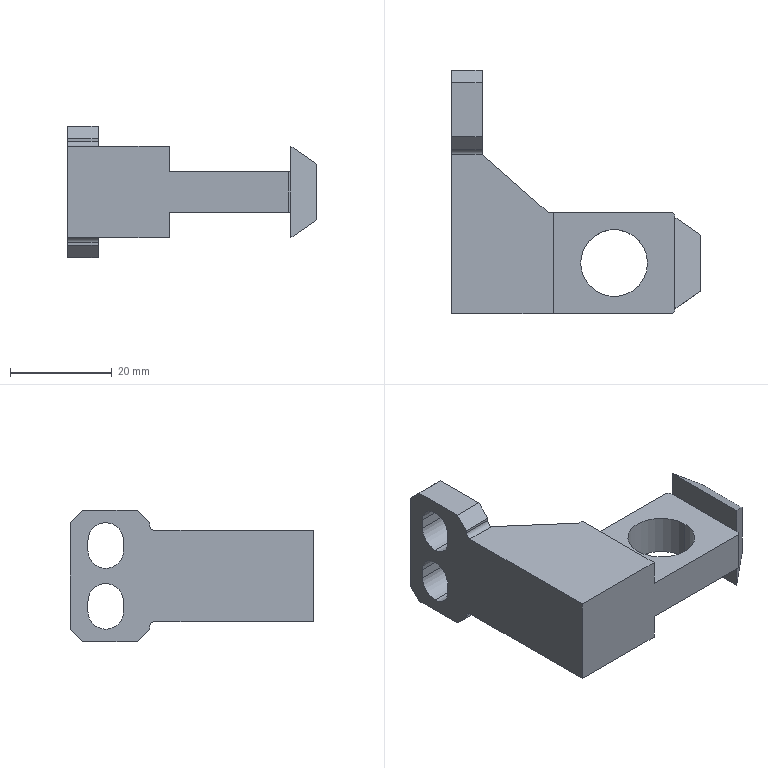Part | SolidWorks | features BaseBody 1 | 1 solid | 51 faces | box 49 x 48 x 26 mm | volume 15129 mm3 | plane 37 | cylinder 14 | commonest cylinder face diameters 7 x6 2 x2 6 x2 8 x2 13.157 x2
STEP:
#1=CARTESIAN_POINT('',(-32.,34.5,-7.));
#2=VERTEX_POINT('',#1);
#3=CARTESIAN_POINT('',(-32.,31.,-10.5));
#4=VERTEX_POINT('',#3);
#5=CARTESIAN_POINT('',(-32.,31.,-7.));
#6=DIRECTION('',(-1.,0.,0.));
#7=DIRECTION('',(0.,0.,-1.));
#8=AXIS2_PLACEMENT_3D('',#5,#6,#7);
#9=CIRCLE('',#8,3.5);
#10=EDGE_CURVE('',#2,#4,#9,.T.);
#11=ORIENTED_EDGE('',*,*,#10,.T.);
#12=CARTESIAN_POINT('',(-26.,31.,-10.5));
#13=VERTEX_POINT('',#12);
#14=CARTESIAN_POINT('',(-26.,31.,-10.5));
#15=DIRECTION('',(1.,0.,0.));
#16=VECTOR('',#15,1000.);
#17=LINE('',#14,#16);
#18=EDGE_CURVE('',#4,#13,#17,.T.);
#19=ORIENTED_EDGE('',*,*,#18,.T.);
#20=CARTESIAN_POINT('',(-26.,34.5,-7.));
#21=VERTEX_POINT('',#20);
#22=CARTESIAN_POINT('',(-26.,31.,-7.));
#23=DIRECTION('',(-1.,0.,0.));
#24=DIRECTION('',(0.,0.,-1.));
#25=AXIS2_PLACEMENT_3D('',#22,#23,#24);
#26=CIRCLE('',#25,3.5);
#27=EDGE_CURVE('',#21,#13,#26,.T.);
#28=ORIENTED_EDGE('',*,*,#27,.F.);
#29=CARTESIAN_POINT('',(-26.,34.5,-7.));
#30=DIRECTION('',(1.,0.,0.));
#31=VECTOR('',#30,1000.);
#32=LINE('',#29,#31);
#33=EDGE_CURVE('',#2,#21,#32,.T.);
#34=ORIENTED_EDGE('',*,*,#33,.F.);
#35=EDGE_LOOP('',(#11,#19,#28,#34));
#36=FACE_OUTER_BOUND('',#35,.T.);
#37=CARTESIAN_POINT('',(-26.,31.,-7.));
#38=DIRECTION('',(1.,0.,0.));
#39=DIRECTION('',(0.,0.,-1.));
#40=AXIS2_PLACEMENT_3D('',#37,#38,#39);
#41=CYLINDRICAL_SURFACE('',#40,3.5);
#42=ADVANCED_FACE('',(#36),#41,.F.);
#43=CARTESIAN_POINT('',(-32.,34.5,5.));
#44=VERTEX_POINT('',#43);
#45=CARTESIAN_POINT('',(-32.,31.,1.5));
#46=VERTEX_POINT('',#45);
#47=CARTESIAN_POINT('',(-32.,31.,5.));
#48=DIRECTION('',(-1.,0.,0.));
#49=DIRECTION('',(0.,0.,-1.));
#50=AXIS2_PLACEMENT_3D('',#47,#48,#49);
#51=CIRCLE('',#50,3.5);
#52=EDGE_CURVE('',#44,#46,#51,.T.);
#53=ORIENTED_EDGE('',*,*,#52,.T.);
#54=CARTESIAN_POINT('',(-26.,31.,1.5));
#55=VERTEX_POINT('',#54);
#56=CARTESIAN_POINT('',(-26.,31.,1.5));
#57=DIRECTION('',(1.,0.,0.));
#58=VECTOR('',#57,1000.);
#59=LINE('',#56,#58);
#60=EDGE_CURVE('',#46,#55,#59,.T.);
#61=ORIENTED_EDGE('',*,*,#60,.T.);
#62=CARTESIAN_POINT('',(-26.,34.5,5.));
#63=VERTEX_POINT('',#62);
#64=CARTESIAN_POINT('',(-26.,31.,5.));
#65=DIRECTION('',(-1.,0.,0.));
#66=DIRECTION('',(0.,0.,-1.));
#67=AXIS2_PLACEMENT_3D('',#64,#65,#66);
#68=CIRCLE('',#67,3.5);
#69=EDGE_CURVE('',#63,#55,#68,.T.);
#70=ORIENTED_EDGE('',*,*,#69,.F.);
#71=CARTESIAN_POINT('',(-26.,34.5,5.));
#72=DIRECTION('',(1.,0.,0.));
#73=VECTOR('',#72,1000.);
#74=LINE('',#71,#73);
#75=EDGE_CURVE('',#44,#63,#74,.T.);
#76=ORIENTED_EDGE('',*,*,#75,.F.);
#77=EDGE_LOOP('',(#53,#61,#70,#76));
#78=FACE_OUTER_BOUND('',#77,.T.);
#79=CARTESIAN_POINT('',(-26.,31.,5.));
#80=DIRECTION('',(1.,0.,0.));
#81=DIRECTION('',(0.,0.,-1.));
#82=AXIS2_PLACEMENT_3D('',#79,#80,#81);
#83=CYLINDRICAL_SURFACE('',#82,3.5);
#84=ADVANCED_FACE('',(#78),#83,.F.);
#85=CARTESIAN_POINT('',(6.579,0.,-4.));
#86=VERTEX_POINT('',#85);
#87=CARTESIAN_POINT('',(-6.579,0.,-4.));
#88=VERTEX_POINT('',#87);
#89=CARTESIAN_POINT('',(0.,0.,-4.));
#90=DIRECTION('',(0.,0.,-1.));
#91=DIRECTION('',(1.,0.,0.));
#92=AXIS2_PLACEMENT_3D('',#89,#90,#91);
#93=CIRCLE('',#92,6.579);
#94=EDGE_CURVE('',#86,#88,#93,.T.);
#95=ORIENTED_EDGE('',*,*,#94,.T.);
#96=CARTESIAN_POINT('',(-6.579,0.,4.));
#97=VERTEX_POINT('',#96);
#98=CARTESIAN_POINT('',(-6.579,0.,-4.));
#99=DIRECTION('',(0.,0.,1.));
#100=VECTOR('',#99,1000.);
#101=LINE('',#98,#100);
#102=EDGE_CURVE('',#88,#97,#101,.T.);
#103=ORIENTED_EDGE('',*,*,#102,.T.);
#104=CARTESIAN_POINT('',(6.579,0.,4.));
#105=VERTEX_POINT('',#104);
#106=CARTESIAN_POINT('',(0.,0.,4.));
#107=DIRECTION('',(0.,0.,-1.));
#108=DIRECTION('',(1.,0.,0.));
#109=AXIS2_PLACEMENT_3D('',#106,#107,#108);
#110=CIRCLE('',#109,6.579);
#111=EDGE_CURVE('',#105,#97,#110,.T.);
#112=ORIENTED_EDGE('',*,*,#111,.F.);
#113=CARTESIAN_POINT('',(6.579,0.,-4.));
#114=DIRECTION('',(0.,0.,1.));
#115=VECTOR('',#114,1000.);
#116=LINE('',#113,#115);
#117=EDGE_CURVE('',#86,#105,#116,.T.);
#118=ORIENTED_EDGE('',*,*,#117,.F.);
#119=EDGE_LOOP('',(#95,#103,#112,#118));
#120=FACE_OUTER_BOUND('',#119,.T.);
#121=CARTESIAN_POINT('',(0.,0.,-4.));
#122=DIRECTION('',(0.,0.,1.));
#123=DIRECTION('',(1.,0.,0.));
#124=AXIS2_PLACEMENT_3D('',#121,#122,#123);
#125=CYLINDRICAL_SURFACE('',#124,6.579);
#126=ADVANCED_FACE('',(#120),#125,.F.);
#127=CARTESIAN_POINT('',(17.,0.,4.));
#128=VERTEX_POINT('',#127);
#129=CARTESIAN_POINT('',(17.,0.,-4.));
#130=VERTEX_POINT('',#129);
#131=CARTESIAN_POINT('',(17.,0.,0.));
#132=DIRECTION('',(1.,0.,0.));
#133=DIRECTION('',(0.,0.,1.));
#134=AXIS2_PLACEMENT_3D('',#131,#132,#133);
#135=CIRCLE('',#134,4.);
#136=EDGE_CURVE('',#128,#130,#135,.T.);
#137=ORIENTED_EDGE('',*,*,#136,.T.);
#138=CARTESIAN_POINT('',(14.,0.,-4.));
#139=VERTEX_POINT('',#138);
#140=CARTESIAN_POINT('',(17.,0.,-4.));
#141=DIRECTION('',(-1.,0.,0.));
#142=VECTOR('',#141,1000.);
#143=LINE('',#140,#142);
#144=EDGE_CURVE('',#130,#139,#143,.T.);
#145=ORIENTED_EDGE('',*,*,#144,.T.);
#146=CARTESIAN_POINT('',(14.,0.,4.));
#147=VERTEX_POINT('',#146);
#148=CARTESIAN_POINT('',(14.,0.,0.));
#149=DIRECTION('',(1.,0.,0.));
#150=DIRECTION('',(0.,0.,1.));
#151=AXIS2_PLACEMENT_3D('',#148,#149,#150);
#152=CIRCLE('',#151,4.);
#153=EDGE_CURVE('',#147,#139,#152,.T.);
#154=ORIENTED_EDGE('',*,*,#153,.F.);
#155=CARTESIAN_POINT('',(17.,0.,4.));
#156=DIRECTION('',(-1.,0.,0.));
#157=VECTOR('',#156,1000.);
#158=LINE('',#155,#157);
#159=EDGE_CURVE('',#128,#147,#158,.T.);
#160=ORIENTED_EDGE('',*,*,#159,.F.);
#161=EDGE_LOOP('',(#137,#145,#154,#160));
#162=FACE_OUTER_BOUND('',#161,.T.);
#163=CARTESIAN_POINT('',(17.,0.,0.));
#164=DIRECTION('',(-1.,0.,0.));
#165=DIRECTION('',(0.,0.,1.));
#166=AXIS2_PLACEMENT_3D('',#163,#164,#165);
#167=CYLINDRICAL_SURFACE('',#166,4.);
#168=ADVANCED_FACE('',(#162),#167,.F.);
#169=CARTESIAN_POINT('',(14.,0.,-3.));
#170=VERTEX_POINT('',#169);
#171=CARTESIAN_POINT('',(14.,0.,3.));
#172=VERTEX_POINT('',#171);
#173=CARTESIAN_POINT('',(14.,0.,0.));
#174=DIRECTION('',(-1.,0.,0.));
#175=DIRECTION('',(0.,0.,1.));
#176=AXIS2_PLACEMENT_3D('',#173,#174,#175);
#177=CIRCLE('',#176,3.);
#178=EDGE_CURVE('',#170,#172,#177,.T.);
#179=ORIENTED_EDGE('',*,*,#178,.F.);
#180=CARTESIAN_POINT('',(9.,0.,-3.));
#181=VERTEX_POINT('',#180);
#182=CARTESIAN_POINT('',(17.,0.,-3.));
#183=DIRECTION('',(-1.,0.,0.));
#184=VECTOR('',#183,1000.);
#185=LINE('',#182,#184);
#186=EDGE_CURVE('',#170,#181,#185,.T.);
#187=ORIENTED_EDGE('',*,*,#186,.T.);
#188=CARTESIAN_POINT('',(9.,0.,3.));
#189=VERTEX_POINT('',#188);
#190=CARTESIAN_POINT('',(9.,0.,0.));
#191=DIRECTION('',(1.,0.,0.));
#192=DIRECTION('',(0.,0.,1.));
#193=AXIS2_PLACEMENT_3D('',#190,#191,#192);
#194=CIRCLE('',#193,3.);
#195=EDGE_CURVE('',#189,#181,#194,.T.);
#196=ORIENTED_EDGE('',*,*,#195,.F.);
#197=CARTESIAN_POINT('',(17.,0.,3.));
#198=DIRECTION('',(-1.,0.,0.));
#199=VECTOR('',#198,1000.);
#200=LINE('',#197,#199);
#201=EDGE_CURVE('',#172,#189,#200,.T.);
#202=ORIENTED_EDGE('',*,*,#201,.F.);
#203=EDGE_LOOP('',(#179,#187,#196,#202));
#204=FACE_OUTER_BOUND('',#203,.T.);
#205=CARTESIAN_POINT('',(17.,0.,0.));
#206=DIRECTION('',(-1.,0.,0.));
#207=DIRECTION('',(0.,0.,1.));
#208=AXIS2_PLACEMENT_3D('',#205,#206,#207);
#209=CYLINDRICAL_SURFACE('',#208,3.);
#210=ADVANCED_FACE('',(#204),#209,.F.);
#211=CARTESIAN_POINT('',(-32.,27.5,-5.));
#212=VERTEX_POINT('',#211);
#213=CARTESIAN_POINT('',(-32.,34.5,-5.));
#214=VERTEX_POINT('',#213);
#215=CARTESIAN_POINT('',(-32.,31.,-5.));
#216=DIRECTION('',(-1.,0.,0.));
#217=DIRECTION('',(0.,0.,-1.));
#218=AXIS2_PLACEMENT_3D('',#215,#216,#217);
#219=CIRCLE('',#218,3.5);
#220=EDGE_CURVE('',#212,#214,#219,.T.);
#221=ORIENTED_EDGE('',*,*,#220,.F.);
#222=CARTESIAN_POINT('',(-32.,27.5,-7.));
#223=VERTEX_POINT('',#222);
#224=CARTESIAN_POINT('',(-32.,27.5,9.));
#225=DIRECTION('',(0.,0.,1.));
#226=VECTOR('',#225,1000.);
#227=LINE('',#224,#226);
#228=EDGE_CURVE('',#223,#212,#227,.T.);
#229=ORIENTED_EDGE('',*,*,#228,.F.);
#230=CARTESIAN_POINT('',(-32.,31.,-7.));
#231=DIRECTION('',(-1.,0.,0.));
#232=DIRECTION('',(0.,0.,-1.));
#233=AXIS2_PLACEMENT_3D('',#230,#231,#232);
#234=CIRCLE('',#233,3.5);
#235=EDGE_CURVE('',#4,#223,#234,.T.);
#236=ORIENTED_EDGE('',*,*,#235,.F.);
#237=ORIENTED_EDGE('',*,*,#10,.F.);
#238=CARTESIAN_POINT('',(-32.,34.5,9.));
#239=DIRECTION('',(0.,0.,-1.));
#240=VECTOR('',#239,1000.);
#241=LINE('',#238,#240);
#242=EDGE_CURVE('',#214,#2,#241,.T.);
#243=ORIENTED_EDGE('',*,*,#242,.F.);
#244=EDGE_LOOP('',(#221,#229,#236,#237,#243));
#245=FACE_BOUND('',#244,.T.);
#246=CARTESIAN_POINT('',(-32.,27.5,7.));
#247=VERTEX_POINT('',#246);
#248=CARTESIAN_POINT('',(-32.,34.5,7.));
#249=VERTEX_POINT('',#248);
#250=CARTESIAN_POINT('',(-32.,31.,7.));
#251=DIRECTION('',(-1.,0.,0.));
#252=DIRECTION('',(0.,0.,-1.));
#253=AXIS2_PLACEMENT_3D('',#250,#251,#252);
#254=CIRCLE('',#253,3.5);
#255=EDGE_CURVE('',#247,#249,#254,.T.);
#256=ORIENTED_EDGE('',*,*,#255,.F.);
#257=CARTESIAN_POINT('',(-32.,27.5,5.));
#258=VERTEX_POINT('',#257);
#259=CARTESIAN_POINT('',(-32.,27.5,9.));
#260=DIRECTION('',(0.,0.,1.));
#261=VECTOR('',#260,1000.);
#262=LINE('',#259,#261);
#263=EDGE_CURVE('',#258,#247,#262,.T.);
#264=ORIENTED_EDGE('',*,*,#263,.F.);
#265=CARTESIAN_POINT('',(-32.,31.,5.));
#266=DIRECTION('',(-1.,0.,0.));
#267=DIRECTION('',(0.,0.,-1.));
#268=AXIS2_PLACEMENT_3D('',#265,#266,#267);
#269=CIRCLE('',#268,3.5);
#270=EDGE_CURVE('',#46,#258,#269,.T.);
#271=ORIENTED_EDGE('',*,*,#270,.F.);
#272=ORIENTED_EDGE('',*,*,#52,.F.);
#273=CARTESIAN_POINT('',(-32.,34.5,9.));
#274=DIRECTION('',(0.,0.,-1.));
#275=VECTOR('',#274,1000.);
#276=LINE('',#273,#275);
#277=EDGE_CURVE('',#249,#44,#276,.T.);
#278=ORIENTED_EDGE('',*,*,#277,.F.);
#279=EDGE_LOOP('',(#256,#264,#271,#272,#278));
#280=FACE_BOUND('',#279,.T.);
#281=CARTESIAN_POINT('',(-32.,-10.,9.));
#282=VERTEX_POINT('',#281);
#283=CARTESIAN_POINT('',(-32.,-10.,-9.));
#284=VERTEX_POINT('',#283);
#285=CARTESIAN_POINT('',(-32.,-10.,9.));
#286=DIRECTION('',(0.,0.,-1.));
#287=VECTOR('',#286,1000.);
#288=LINE('',#285,#287);
#289=EDGE_CURVE('',#282,#284,#288,.T.);
#290=ORIENTED_EDGE('',*,*,#289,.F.);
#291=CARTESIAN_POINT('',(-32.,21.32,9.));
#292=VERTEX_POINT('',#291);
#293=CARTESIAN_POINT('',(-32.,21.32,9.));
#294=DIRECTION('',(0.,-1.,0.));
#295=VECTOR('',#294,1000.);
#296=LINE('',#293,#295);
#297=EDGE_CURVE('',#292,#282,#296,.T.);
#298=ORIENTED_EDGE('',*,*,#297,.F.);
#299=CARTESIAN_POINT('',(-32.,22.32,10.));
#300=VERTEX_POINT('',#299);
#301=CARTESIAN_POINT('',(-32.,21.32,10.));
#302=DIRECTION('',(1.,0.,0.));
#303=DIRECTION('',(0.,0.,-1.));
#304=AXIS2_PLACEMENT_3D('',#301,#302,#303);
#305=CIRCLE('',#304,1.);
#306=EDGE_CURVE('',#292,#300,#305,.T.);
#307=ORIENTED_EDGE('',*,*,#306,.T.);
#308=CARTESIAN_POINT('',(-32.,22.32,10.5));
#309=VERTEX_POINT('',#308);
#310=CARTESIAN_POINT('',(-32.,22.32,10.5));
#311=DIRECTION('',(0.,0.,1.));
#312=VECTOR('',#311,1000.);
#313=LINE('',#310,#312);
#314=EDGE_CURVE('',#300,#309,#313,.T.);
#315=ORIENTED_EDGE('',*,*,#314,.T.);
#316=CARTESIAN_POINT('',(-32.,24.82,13.));
#317=VERTEX_POINT('',#316);
#318=CARTESIAN_POINT('',(-32.,24.82,13.));
#319=DIRECTION('',(0.,-0.7071,-0.7071));
#320=VECTOR('',#319,1000.);
#321=LINE('',#318,#320);
#322=EDGE_CURVE('',#317,#309,#321,.T.);
#323=ORIENTED_EDGE('',*,*,#322,.F.);
#324=CARTESIAN_POINT('',(-32.,35.5,13.));
#325=VERTEX_POINT('',#324);
#326=CARTESIAN_POINT('',(-32.,21.32,13.));
#327=DIRECTION('',(0.,-1.,0.));
#328=VECTOR('',#327,1000.);
#329=LINE('',#326,#328);
#330=EDGE_CURVE('',#325,#317,#329,.T.);
#331=ORIENTED_EDGE('',*,*,#330,.F.);
#332=CARTESIAN_POINT('',(-32.,38.,10.5));
#333=VERTEX_POINT('',#332);
#334=CARTESIAN_POINT('',(-32.,38.,10.5));
#335=DIRECTION('',(0.,-0.7071,0.7071));
#336=VECTOR('',#335,1000.);
#337=LINE('',#334,#336);
#338=EDGE_CURVE('',#333,#325,#337,.T.);
#339=ORIENTED_EDGE('',*,*,#338,.F.);
#340=CARTESIAN_POINT('',(-32.,38.,-10.5));
#341=VERTEX_POINT('',#340);
#342=CARTESIAN_POINT('',(-32.,38.,9.));
#343=DIRECTION('',(0.,0.,1.));
#344=VECTOR('',#343,1000.);
#345=LINE('',#342,#344);
#346=EDGE_CURVE('',#341,#333,#345,.T.);
#347=ORIENTED_EDGE('',*,*,#346,.F.);
#348=CARTESIAN_POINT('',(-32.,35.5,-13.));
#349=VERTEX_POINT('',#348);
#350=CARTESIAN_POINT('',(-32.,35.5,-13.));
#351=DIRECTION('',(0.,0.7071,0.7071));
#352=VECTOR('',#351,1000.);
#353=LINE('',#350,#352);
#354=EDGE_CURVE('',#349,#341,#353,.T.);
#355=ORIENTED_EDGE('',*,*,#354,.F.);
#356=CARTESIAN_POINT('',(-32.,24.82,-13.));
#357=VERTEX_POINT('',#356);
#358=CARTESIAN_POINT('',(-32.,21.32,-13.));
#359=DIRECTION('',(0.,1.,0.));
#360=VECTOR('',#359,1000.);
#361=LINE('',#358,#360);
#362=EDGE_CURVE('',#357,#349,#361,.T.);
#363=ORIENTED_EDGE('',*,*,#362,.F.);
#364=CARTESIAN_POINT('',(-32.,22.32,-10.5));
#365=VERTEX_POINT('',#364);
#366=CARTESIAN_POINT('',(-32.,22.32,-10.5));
#367=DIRECTION('',(0.,0.7071,-0.7071));
#368=VECTOR('',#367,1000.);
#369=LINE('',#366,#368);
#370=EDGE_CURVE('',#365,#357,#369,.T.);
#371=ORIENTED_EDGE('',*,*,#370,.F.);
#372=CARTESIAN_POINT('',(-32.,22.32,-10.));
#373=VERTEX_POINT('',#372);
#374=CARTESIAN_POINT('',(-32.,22.32,-10.));
#375=DIRECTION('',(0.,0.,1.));
#376=VECTOR('',#375,1000.);
#377=LINE('',#374,#376);
#378=EDGE_CURVE('',#365,#373,#377,.T.);
#379=ORIENTED_EDGE('',*,*,#378,.T.);
#380=CARTESIAN_POINT('',(-32.,21.32,-9.));
#381=VERTEX_POINT('',#380);
#382=CARTESIAN_POINT('',(-32.,21.32,-10.));
#383=DIRECTION('',(1.,0.,0.));
#384=DIRECTION('',(0.,0.,-1.));
#385=AXIS2_PLACEMENT_3D('',#382,#383,#384);
#386=CIRCLE('',#385,1.);
#387=EDGE_CURVE('',#373,#381,#386,.T.);
#388=ORIENTED_EDGE('',*,*,#387,.T.);
#389=CARTESIAN_POINT('',(-32.,21.32,-9.));
#390=DIRECTION('',(0.,1.,0.));
#391=VECTOR('',#390,1000.);
#392=LINE('',#389,#391);
#393=EDGE_CURVE('',#284,#381,#392,.T.);
#394=ORIENTED_EDGE('',*,*,#393,.F.);
#395=EDGE_LOOP('',(#290,#298,#307,#315,#323,#331,#339,#347,#355,#363,#371,#379,#388,#394));
#396=FACE_OUTER_BOUND('',#395,.T.);
#397=CARTESIAN_POINT('',(-32.,21.32,9.));
#398=DIRECTION('',(1.,0.,0.));
#399=DIRECTION('',(0.,0.,-1.));
#400=AXIS2_PLACEMENT_3D('',#397,#398,#399);
#401=PLANE('',#400);
#402=ADVANCED_FACE('',(#245,#280,#396),#401,.F.);
#403=CARTESIAN_POINT('',(-26.,34.5,-5.));
#404=VERTEX_POINT('',#403);
#405=CARTESIAN_POINT('',(-26.,34.5,-7.));
#406=DIRECTION('',(0.,0.,1.));
#407=VECTOR('',#406,1000.);
#408=LINE('',#405,#407);
#409=EDGE_CURVE('',#21,#404,#408,.T.);
#410=ORIENTED_EDGE('',*,*,#409,.T.);
#411=CARTESIAN_POINT('',(-26.,34.5,-5.));
#412=DIRECTION('',(-1.,0.,0.));
#413=VECTOR('',#412,1000.);
#414=LINE('',#411,#413);
#415=EDGE_CURVE('',#404,#214,#414,.T.);
#416=ORIENTED_EDGE('',*,*,#415,.T.);
#417=ORIENTED_EDGE('',*,*,#242,.T.);
#418=ORIENTED_EDGE('',*,*,#33,.T.);
#419=EDGE_LOOP('',(#410,#416,#417,#418));
#420=FACE_OUTER_BOUND('',#419,.T.);
#421=CARTESIAN_POINT('',(-26.,34.5,-7.));
#422=DIRECTION('',(0.,-1.,0.));
#423=DIRECTION('',(0.,0.,-1.));
#424=AXIS2_PLACEMENT_3D('',#421,#422,#423);
#425=PLANE('',#424);
#426=ADVANCED_FACE('',(#420),#425,.T.);
#427=ORIENTED_EDGE('',*,*,#415,.F.);
#428=CARTESIAN_POINT('',(-26.,27.5,-5.));
#429=VERTEX_POINT('',#428);
#430=CARTESIAN_POINT('',(-26.,31.,-5.));
#431=DIRECTION('',(-1.,0.,0.));
#432=DIRECTION('',(0.,0.,-1.));
#433=AXIS2_PLACEMENT_3D('',#430,#431,#432);
#434=CIRCLE('',#433,3.5);
#435=EDGE_CURVE('',#429,#404,#434,.T.);
#436=ORIENTED_EDGE('',*,*,#435,.F.);
#437=CARTESIAN_POINT('',(-26.,27.5,-5.));
#438=DIRECTION('',(1.,0.,0.));
#439=VECTOR('',#438,1000.);
#440=LINE('',#437,#439);
#441=EDGE_CURVE('',#212,#429,#440,.T.);
#442=ORIENTED_EDGE('',*,*,#441,.F.);
#443=ORIENTED_EDGE('',*,*,#220,.T.);
#444=EDGE_LOOP('',(#427,#436,#442,#443));
#445=FACE_OUTER_BOUND('',#444,.T.);
#446=CARTESIAN_POINT('',(-26.,31.,-5.));
#447=DIRECTION('',(1.,0.,0.));
#448=DIRECTION('',(0.,0.,-1.));
#449=AXIS2_PLACEMENT_3D('',#446,#447,#448);
#450=CYLINDRICAL_SURFACE('',#449,3.5);
#451=ADVANCED_FACE('',(#445),#450,.F.);
#452=CARTESIAN_POINT('',(-26.,27.5,-7.));
#453=VERTEX_POINT('',#452);
#454=CARTESIAN_POINT('',(-26.,27.5,-5.));
#455=DIRECTION('',(0.,0.,-1.));
#456=VECTOR('',#455,1000.);
#457=LINE('',#454,#456);
#458=EDGE_CURVE('',#429,#453,#457,.T.);
#459=ORIENTED_EDGE('',*,*,#458,.T.);
#460=CARTESIAN_POINT('',(-26.,27.5,-7.));
#461=DIRECTION('',(-1.,0.,0.));
#462=VECTOR('',#461,1000.);
#463=LINE('',#460,#462);
#464=EDGE_CURVE('',#453,#223,#463,.T.);
#465=ORIENTED_EDGE('',*,*,#464,.T.);
#466=ORIENTED_EDGE('',*,*,#228,.T.);
#467=ORIENTED_EDGE('',*,*,#441,.T.);
#468=EDGE_LOOP('',(#459,#465,#466,#467));
#469=FACE_OUTER_BOUND('',#468,.T.);
#470=CARTESIAN_POINT('',(-26.,27.5,-5.));
#471=DIRECTION('',(0.,1.,0.));
#472=DIRECTION('',(0.,0.,1.));
#473=AXIS2_PLACEMENT_3D('',#470,#471,#472);
#474=PLANE('',#473);
#475=ADVANCED_FACE('',(#469),#474,.T.);
#476=ORIENTED_EDGE('',*,*,#18,.F.);
#477=ORIENTED_EDGE('',*,*,#235,.T.);
#478=ORIENTED_EDGE('',*,*,#464,.F.);
#479=CARTESIAN_POINT('',(-26.,31.,-7.));
#480=DIRECTION('',(-1.,0.,0.));
#481=DIRECTION('',(0.,0.,-1.));
#482=AXIS2_PLACEMENT_3D('',#479,#480,#481);
#483=CIRCLE('',#482,3.5);
#484=EDGE_CURVE('',#13,#453,#483,.T.);
#485=ORIENTED_EDGE('',*,*,#484,.F.);
#486=EDGE_LOOP('',(#476,#477,#478,#485));
#487=FACE_OUTER_BOUND('',#486,.T.);
#488=CARTESIAN_POINT('',(-26.,31.,-7.));
#489=DIRECTION('',(1.,0.,0.));
#490=DIRECTION('',(0.,0.,-1.));
#491=AXIS2_PLACEMENT_3D('',#488,#489,#490);
#492=CYLINDRICAL_SURFACE('',#491,3.5);
#493=ADVANCED_FACE('',(#487),#492,.F.);
#494=CARTESIAN_POINT('',(-26.,34.5,7.));
#495=VERTEX_POINT('',#494);
#496=CARTESIAN_POINT('',(-26.,34.5,5.));
#497=DIRECTION('',(0.,0.,1.));
#498=VECTOR('',#497,1000.);
#499=LINE('',#496,#498);
#500=EDGE_CURVE('',#63,#495,#499,.T.);
#501=ORIENTED_EDGE('',*,*,#500,.T.);
#502=CARTESIAN_POINT('',(-26.,34.5,7.));
#503=DIRECTION('',(-1.,0.,0.));
#504=VECTOR('',#503,1000.);
#505=LINE('',#502,#504);
#506=EDGE_CURVE('',#495,#249,#505,.T.);
#507=ORIENTED_EDGE('',*,*,#506,.T.);
#508=ORIENTED_EDGE('',*,*,#277,.T.);
#509=ORIENTED_EDGE('',*,*,#75,.T.);
#510=EDGE_LOOP('',(#501,#507,#508,#509));
#511=FACE_OUTER_BOUND('',#510,.T.);
#512=CARTESIAN_POINT('',(-26.,34.5,5.));
#513=DIRECTION('',(0.,-1.,0.));
#514=DIRECTION('',(0.,0.,-1.));
#515=AXIS2_PLACEMENT_3D('',#512,#513,#514);
#516=PLANE('',#515);
#517=ADVANCED_FACE('',(#511),#516,.T.);
#518=ORIENTED_EDGE('',*,*,#506,.F.);
#519=CARTESIAN_POINT('',(-26.,27.5,7.));
#520=VERTEX_POINT('',#519);
#521=CARTESIAN_POINT('',(-26.,31.,7.));
#522=DIRECTION('',(-1.,0.,0.));
#523=DIRECTION('',(0.,0.,-1.));
#524=AXIS2_PLACEMENT_3D('',#521,#522,#523);
#525=CIRCLE('',#524,3.5);
#526=EDGE_CURVE('',#520,#495,#525,.T.);
#527=ORIENTED_EDGE('',*,*,#526,.F.);
#528=CARTESIAN_POINT('',(-26.,27.5,7.));
#529=DIRECTION('',(1.,0.,0.));
#530=VECTOR('',#529,1000.);
#531=LINE('',#528,#530);
#532=EDGE_CURVE('',#247,#520,#531,.T.);
#533=ORIENTED_EDGE('',*,*,#532,.F.);
#534=ORIENTED_EDGE('',*,*,#255,.T.);
#535=EDGE_LOOP('',(#518,#527,#533,#534));
#536=FACE_OUTER_BOUND('',#535,.T.);
#537=CARTESIAN_POINT('',(-26.,31.,7.));
#538=DIRECTION('',(1.,0.,0.));
#539=DIRECTION('',(0.,0.,-1.));
#540=AXIS2_PLACEMENT_3D('',#537,#538,#539);
#541=CYLINDRICAL_SURFACE('',#540,3.5);
#542=ADVANCED_FACE('',(#536),#541,.F.);
#543=CARTESIAN_POINT('',(-26.,27.5,5.));
#544=VERTEX_POINT('',#543);
#545=CARTESIAN_POINT('',(-26.,27.5,7.));
#546=DIRECTION('',(0.,0.,-1.));
#547=VECTOR('',#546,1000.);
#548=LINE('',#545,#547);
#549=EDGE_CURVE('',#520,#544,#548,.T.);
#550=ORIENTED_EDGE('',*,*,#549,.T.);
#551=CARTESIAN_POINT('',(-26.,27.5,5.));
#552=DIRECTION('',(-1.,0.,0.));
#553=VECTOR('',#552,1000.);
#554=LINE('',#551,#553);
#555=EDGE_CURVE('',#544,#258,#554,.T.);
#556=ORIENTED_EDGE('',*,*,#555,.T.);
#557=ORIENTED_EDGE('',*,*,#263,.T.);
#558=ORIENTED_EDGE('',*,*,#532,.T.);
#559=EDGE_LOOP('',(#550,#556,#557,#558));
#560=FACE_OUTER_BOUND('',#559,.T.);
#561=CARTESIAN_POINT('',(-26.,27.5,7.));
#562=DIRECTION('',(0.,1.,0.));
#563=DIRECTION('',(0.,0.,1.));
#564=AXIS2_PLACEMENT_3D('',#561,#562,#563);
#565=PLANE('',#564);
#566=ADVANCED_FACE('',(#560),#565,.T.);
#567=ORIENTED_EDGE('',*,*,#60,.F.);
#568=ORIENTED_EDGE('',*,*,#270,.T.);
#569=ORIENTED_EDGE('',*,*,#555,.F.);
#570=CARTESIAN_POINT('',(-26.,31.,5.));
#571=DIRECTION('',(-1.,0.,0.));
#572=DIRECTION('',(0.,0.,-1.));
#573=AXIS2_PLACEMENT_3D('',#570,#571,#572);
#574=CIRCLE('',#573,3.5);
#575=EDGE_CURVE('',#55,#544,#574,.T.);
#576=ORIENTED_EDGE('',*,*,#575,.F.);
#577=EDGE_LOOP('',(#567,#568,#569,#576));
#578=FACE_OUTER_BOUND('',#577,.T.);
#579=CARTESIAN_POINT('',(-26.,31.,5.));
#580=DIRECTION('',(1.,0.,0.));
#581=DIRECTION('',(0.,0.,-1.));
#582=AXIS2_PLACEMENT_3D('',#579,#580,#581);
#583=CYLINDRICAL_SURFACE('',#582,3.5);
#584=ADVANCED_FACE('',(#578),#583,.F.);
#585=CARTESIAN_POINT('',(-26.,21.32,-9.));
#586=VERTEX_POINT('',#585);
#587=CARTESIAN_POINT('',(0.,21.32,-9.));
#588=DIRECTION('',(-1.,0.,0.));
#589=VECTOR('',#588,1000.);
#590=LINE('',#587,#589);
#591=EDGE_CURVE('',#586,#381,#590,.T.);
#592=ORIENTED_EDGE('',*,*,#591,.F.);
#593=CARTESIAN_POINT('',(-13.,10.,-9.));
#594=VERTEX_POINT('',#593);
#595=CARTESIAN_POINT('',(-13.,10.,-9.));
#596=DIRECTION('',(-0.7542,0.6567,0.));
#597=VECTOR('',#596,1000.);
#598=LINE('',#595,#597);
#599=EDGE_CURVE('',#594,#586,#598,.T.);
#600=ORIENTED_EDGE('',*,*,#599,.F.);
#601=CARTESIAN_POINT('',(-12.,10.,-9.));
#602=VERTEX_POINT('',#601);
#603=CARTESIAN_POINT('',(11.5,10.,-9.));
#604=DIRECTION('',(1.,0.,0.));
#605=VECTOR('',#604,1000.);
#606=LINE('',#603,#605);
#607=EDGE_CURVE('',#594,#602,#606,.T.);
#608=ORIENTED_EDGE('',*,*,#607,.T.);
#609=CARTESIAN_POINT('',(-12.,-10.,-9.));
#610=VERTEX_POINT('',#609);
#611=CARTESIAN_POINT('',(-12.,0.,-9.));
#612=DIRECTION('',(0.,1.,0.));
#613=VECTOR('',#612,1000.);
#614=LINE('',#611,#613);
#615=EDGE_CURVE('',#610,#602,#614,.T.);
#616=ORIENTED_EDGE('',*,*,#615,.F.);
#617=CARTESIAN_POINT('',(0.,-10.,-9.));
#618=DIRECTION('',(1.,0.,0.));
#619=VECTOR('',#618,1000.);
#620=LINE('',#617,#619);
#621=EDGE_CURVE('',#284,#610,#620,.T.);
#622=ORIENTED_EDGE('',*,*,#621,.F.);
#623=ORIENTED_EDGE('',*,*,#393,.T.);
#624=EDGE_LOOP('',(#592,#600,#608,#616,#622,#623));
#625=FACE_OUTER_BOUND('',#624,.T.);
#626=CARTESIAN_POINT('',(0.,0.,-9.));
#627=DIRECTION('',(0.,0.,1.));
#628=DIRECTION('',(1.,0.,0.));
#629=AXIS2_PLACEMENT_3D('',#626,#627,#628);
#630=PLANE('',#629);
#631=ADVANCED_FACE('',(#625),#630,.F.);
#632=CARTESIAN_POINT('',(11.5,-10.,4.));
#633=VERTEX_POINT('',#632);
#634=CARTESIAN_POINT('',(11.5,-10.,-4.));
#635=VERTEX_POINT('',#634);
#636=CARTESIAN_POINT('',(11.5,-10.,4.));
#637=DIRECTION('',(0.,0.,-1.));
#638=VECTOR('',#637,1000.);
#639=LINE('',#636,#638);
#640=EDGE_CURVE('',#633,#635,#639,.T.);
#641=ORIENTED_EDGE('',*,*,#640,.F.);
#642=CARTESIAN_POINT('',(-12.,-10.,4.));
#643=VERTEX_POINT('',#642);
#644=CARTESIAN_POINT('',(-12.,-10.,4.));
#645=DIRECTION('',(1.,0.,0.));
#646=VECTOR('',#645,1000.);
#647=LINE('',#644,#646);
#648=EDGE_CURVE('',#643,#633,#647,.T.);
#649=ORIENTED_EDGE('',*,*,#648,.F.);
#650=CARTESIAN_POINT('',(-12.,-10.,9.));
#651=VERTEX_POINT('',#650);
#652=CARTESIAN_POINT('',(-12.,-10.,4.));
#653=DIRECTION('',(0.,0.,-1.));
#654=VECTOR('',#653,1000.);
#655=LINE('',#652,#654);
#656=EDGE_CURVE('',#651,#643,#655,.T.);
#657=ORIENTED_EDGE('',*,*,#656,.F.);
#658=CARTESIAN_POINT('',(-12.,-10.,9.));
#659=DIRECTION('',(1.,0.,0.));
#660=VECTOR('',#659,1000.);
#661=LINE('',#658,#660);
#662=EDGE_CURVE('',#282,#651,#661,.T.);
#663=ORIENTED_EDGE('',*,*,#662,.F.);
#664=ORIENTED_EDGE('',*,*,#289,.T.);
#665=ORIENTED_EDGE('',*,*,#621,.T.);
#666=CARTESIAN_POINT('',(-12.,-10.,-4.));
#667=VERTEX_POINT('',#666);
#668=CARTESIAN_POINT('',(-12.,-10.,4.));
#669=DIRECTION('',(0.,0.,-1.));
#670=VECTOR('',#669,1000.);
#671=LINE('',#668,#670);
#672=EDGE_CURVE('',#667,#610,#671,.T.);
#673=ORIENTED_EDGE('',*,*,#672,.F.);
#674=CARTESIAN_POINT('',(-12.,-10.,-4.));
#675=DIRECTION('',(-1.,0.,0.));
#676=VECTOR('',#675,1000.);
#677=LINE('',#674,#676);
#678=EDGE_CURVE('',#635,#667,#677,.T.);
#679=ORIENTED_EDGE('',*,*,#678,.F.);
#680=EDGE_LOOP('',(#641,#649,#657,#663,#664,#665,#673,#679));
#681=FACE_OUTER_BOUND('',#680,.T.);
#682=CARTESIAN_POINT('',(-12.,-10.,4.));
#683=DIRECTION('',(0.,1.,0.));
#684=DIRECTION('',(0.,0.,1.));
#685=AXIS2_PLACEMENT_3D('',#682,#683,#684);
#686=PLANE('',#685);
#687=ADVANCED_FACE('',(#681),#686,.F.);
#688=CARTESIAN_POINT('',(-13.,10.,9.));
#689=VERTEX_POINT('',#688);
#690=CARTESIAN_POINT('',(-26.,21.32,9.));
#691=VERTEX_POINT('',#690);
#692=CARTESIAN_POINT('',(-13.,10.,9.));
#693=DIRECTION('',(-0.7542,0.6567,0.));
#694=VECTOR('',#693,1000.);
#695=LINE('',#692,#694);
#696=EDGE_CURVE('',#689,#691,#695,.T.);
#697=ORIENTED_EDGE('',*,*,#696,.T.);
#698=CARTESIAN_POINT('',(0.,21.32,9.));
#699=DIRECTION('',(-1.,0.,0.));
#700=VECTOR('',#699,1000.);
#701=LINE('',#698,#700);
#702=EDGE_CURVE('',#691,#292,#701,.T.);
#703=ORIENTED_EDGE('',*,*,#702,.T.);
#704=ORIENTED_EDGE('',*,*,#297,.T.);
#705=ORIENTED_EDGE('',*,*,#662,.T.);
#706=CARTESIAN_POINT('',(-12.,10.,9.));
#707=VERTEX_POINT('',#706);
#708=CARTESIAN_POINT('',(-12.,0.,9.));
#709=DIRECTION('',(0.,1.,0.));
#710=VECTOR('',#709,1000.);
#711=LINE('',#708,#710);
#712=EDGE_CURVE('',#651,#707,#711,.T.);
#713=ORIENTED_EDGE('',*,*,#712,.T.);
#714=CARTESIAN_POINT('',(11.5,10.,9.));
#715=DIRECTION('',(-1.,0.,0.));
#716=VECTOR('',#715,1000.);
#717=LINE('',#714,#716);
#718=EDGE_CURVE('',#707,#689,#717,.T.);
#719=ORIENTED_EDGE('',*,*,#718,.T.);
#720=EDGE_LOOP('',(#697,#703,#704,#705,#713,#719));
#721=FACE_OUTER_BOUND('',#720,.T.);
#722=CARTESIAN_POINT('',(0.,0.,9.));
#723=DIRECTION('',(0.,0.,1.));
#724=DIRECTION('',(1.,0.,0.));
#725=AXIS2_PLACEMENT_3D('',#722,#723,#724);
#726=PLANE('',#725);
#727=ADVANCED_FACE('',(#721),#726,.T.);
#728=CARTESIAN_POINT('',(-26.,22.32,10.5));
#729=VERTEX_POINT('',#728);
#730=CARTESIAN_POINT('',(-26.,22.32,10.5));
#731=DIRECTION('',(-1.,0.,0.));
#732=VECTOR('',#731,1000.);
#733=LINE('',#730,#732);
#734=EDGE_CURVE('',#729,#309,#733,.T.);
#735=ORIENTED_EDGE('',*,*,#734,.F.);
#736=CARTESIAN_POINT('',(-26.,24.82,13.));
#737=VERTEX_POINT('',#736);
#738=CARTESIAN_POINT('',(-26.,24.82,13.));
#739=DIRECTION('',(0.,-0.7071,-0.7071));
#740=VECTOR('',#739,1000.);
#741=LINE('',#738,#740);
#742=EDGE_CURVE('',#737,#729,#741,.T.);
#743=ORIENTED_EDGE('',*,*,#742,.F.);
#744=CARTESIAN_POINT('',(-26.,24.82,13.));
#745=DIRECTION('',(1.,0.,0.));
#746=VECTOR('',#745,1000.);
#747=LINE('',#744,#746);
#748=EDGE_CURVE('',#317,#737,#747,.T.);
#749=ORIENTED_EDGE('',*,*,#748,.F.);
#750=ORIENTED_EDGE('',*,*,#322,.T.);
#751=EDGE_LOOP('',(#735,#743,#749,#750));
#752=FACE_OUTER_BOUND('',#751,.T.);
#753=CARTESIAN_POINT('',(-26.,24.82,13.));
#754=DIRECTION('',(0.,0.7071,-0.7071));
#755=DIRECTION('',(0.,0.7071,0.7071));
#756=AXIS2_PLACEMENT_3D('',#753,#754,#755);
#757=PLANE('',#756);
#758=ADVANCED_FACE('',(#752),#757,.F.);
#759=ORIENTED_EDGE('',*,*,#748,.T.);
#760=CARTESIAN_POINT('',(-26.,35.5,13.));
#761=VERTEX_POINT('',#760);
#762=CARTESIAN_POINT('',(-26.,35.5,13.));
#763=DIRECTION('',(0.,-1.,0.));
#764=VECTOR('',#763,1000.);
#765=LINE('',#762,#764);
#766=EDGE_CURVE('',#761,#737,#765,.T.);
#767=ORIENTED_EDGE('',*,*,#766,.F.);
#768=CARTESIAN_POINT('',(-26.,35.5,13.));
#769=DIRECTION('',(1.,0.,0.));
#770=VECTOR('',#769,1000.);
#771=LINE('',#768,#770);
#772=EDGE_CURVE('',#325,#761,#771,.T.);
#773=ORIENTED_EDGE('',*,*,#772,.F.);
#774=ORIENTED_EDGE('',*,*,#330,.T.);
#775=EDGE_LOOP('',(#759,#767,#773,#774));
#776=FACE_OUTER_BOUND('',#775,.T.);
#777=CARTESIAN_POINT('',(-26.,35.5,13.));
#778=DIRECTION('',(0.,0.,-1.));
#779=DIRECTION('',(-1.,0.,0.));
#780=AXIS2_PLACEMENT_3D('',#777,#778,#779);
#781=PLANE('',#780);
#782=ADVANCED_FACE('',(#776),#781,.F.);
#783=ORIENTED_EDGE('',*,*,#772,.T.);
#784=CARTESIAN_POINT('',(-26.,38.,10.5));
#785=VERTEX_POINT('',#784);
#786=CARTESIAN_POINT('',(-26.,38.,10.5));
#787=DIRECTION('',(0.,-0.7071,0.7071));
#788=VECTOR('',#787,1000.);
#789=LINE('',#786,#788);
#790=EDGE_CURVE('',#785,#761,#789,.T.);
#791=ORIENTED_EDGE('',*,*,#790,.F.);
#792=CARTESIAN_POINT('',(-26.,38.,10.5));
#793=DIRECTION('',(1.,0.,0.));
#794=VECTOR('',#793,1000.);
#795=LINE('',#792,#794);
#796=EDGE_CURVE('',#333,#785,#795,.T.);
#797=ORIENTED_EDGE('',*,*,#796,.F.);
#798=ORIENTED_EDGE('',*,*,#338,.T.);
#799=EDGE_LOOP('',(#783,#791,#797,#798));
#800=FACE_OUTER_BOUND('',#799,.T.);
#801=CARTESIAN_POINT('',(-26.,38.,10.5));
#802=DIRECTION('',(0.,-0.7071,-0.7071));
#803=DIRECTION('',(0.,0.7071,-0.7071));
#804=AXIS2_PLACEMENT_3D('',#801,#802,#803);
#805=PLANE('',#804);
#806=ADVANCED_FACE('',(#800),#805,.F.);
#807=ORIENTED_EDGE('',*,*,#796,.T.);
#808=CARTESIAN_POINT('',(-26.,38.,-10.5));
#809=VERTEX_POINT('',#808);
#810=CARTESIAN_POINT('',(-26.,38.,-10.5));
#811=DIRECTION('',(0.,0.,1.));
#812=VECTOR('',#811,1000.);
#813=LINE('',#810,#812);
#814=EDGE_CURVE('',#809,#785,#813,.T.);
#815=ORIENTED_EDGE('',*,*,#814,.F.);
#816=CARTESIAN_POINT('',(-26.,38.,-10.5));
#817=DIRECTION('',(1.,0.,0.));
#818=VECTOR('',#817,1000.);
#819=LINE('',#816,#818);
#820=EDGE_CURVE('',#341,#809,#819,.T.);
#821=ORIENTED_EDGE('',*,*,#820,.F.);
#822=ORIENTED_EDGE('',*,*,#346,.T.);
#823=EDGE_LOOP('',(#807,#815,#821,#822));
#824=FACE_OUTER_BOUND('',#823,.T.);
#825=CARTESIAN_POINT('',(-26.,38.,-10.5));
#826=DIRECTION('',(0.,-1.,0.));
#827=DIRECTION('',(0.,0.,-1.));
#828=AXIS2_PLACEMENT_3D('',#825,#826,#827);
#829=PLANE('',#828);
#830=ADVANCED_FACE('',(#824),#829,.F.);
#831=ORIENTED_EDGE('',*,*,#820,.T.);
#832=CARTESIAN_POINT('',(-26.,35.5,-13.));
#833=VERTEX_POINT('',#832);
#834=CARTESIAN_POINT('',(-26.,35.5,-13.));
#835=DIRECTION('',(0.,0.7071,0.7071));
#836=VECTOR('',#835,1000.);
#837=LINE('',#834,#836);
#838=EDGE_CURVE('',#833,#809,#837,.T.);
#839=ORIENTED_EDGE('',*,*,#838,.F.);
#840=CARTESIAN_POINT('',(-26.,35.5,-13.));
#841=DIRECTION('',(1.,0.,0.));
#842=VECTOR('',#841,1000.);
#843=LINE('',#840,#842);
#844=EDGE_CURVE('',#349,#833,#843,.T.);
#845=ORIENTED_EDGE('',*,*,#844,.F.);
#846=ORIENTED_EDGE('',*,*,#354,.T.);
#847=EDGE_LOOP('',(#831,#839,#845,#846));
#848=FACE_OUTER_BOUND('',#847,.T.);
#849=CARTESIAN_POINT('',(-26.,35.5,-13.));
#850=DIRECTION('',(0.,-0.7071,0.7071));
#851=DIRECTION('',(0.,-0.7071,-0.7071));
#852=AXIS2_PLACEMENT_3D('',#849,#850,#851);
#853=PLANE('',#852);
#854=ADVANCED_FACE('',(#848),#853,.F.);
#855=ORIENTED_EDGE('',*,*,#844,.T.);
#856=CARTESIAN_POINT('',(-26.,24.82,-13.));
#857=VERTEX_POINT('',#856);
#858=CARTESIAN_POINT('',(-26.,24.82,-13.));
#859=DIRECTION('',(0.,1.,0.));
#860=VECTOR('',#859,1000.);
#861=LINE('',#858,#860);
#862=EDGE_CURVE('',#857,#833,#861,.T.);
#863=ORIENTED_EDGE('',*,*,#862,.F.);
#864=CARTESIAN_POINT('',(-26.,24.82,-13.));
#865=DIRECTION('',(1.,0.,0.));
#866=VECTOR('',#865,1000.);
#867=LINE('',#864,#866);
#868=EDGE_CURVE('',#357,#857,#867,.T.);
#869=ORIENTED_EDGE('',*,*,#868,.F.);
#870=ORIENTED_EDGE('',*,*,#362,.T.);
#871=EDGE_LOOP('',(#855,#863,#869,#870));
#872=FACE_OUTER_BOUND('',#871,.T.);
#873=CARTESIAN_POINT('',(-26.,24.82,-13.));
#874=DIRECTION('',(0.,0.,1.));
#875=DIRECTION('',(1.,0.,0.));
#876=AXIS2_PLACEMENT_3D('',#873,#874,#875);
#877=PLANE('',#876);
#878=ADVANCED_FACE('',(#872),#877,.F.);
#879=ORIENTED_EDGE('',*,*,#868,.T.);
#880=CARTESIAN_POINT('',(-26.,22.32,-10.5));
#881=VERTEX_POINT('',#880);
#882=CARTESIAN_POINT('',(-26.,22.32,-10.5));
#883=DIRECTION('',(0.,0.7071,-0.7071));
#884=VECTOR('',#883,1000.);
#885=LINE('',#882,#884);
#886=EDGE_CURVE('',#881,#857,#885,.T.);
#887=ORIENTED_EDGE('',*,*,#886,.F.);
#888=CARTESIAN_POINT('',(-26.,22.32,-10.5));
#889=DIRECTION('',(1.,0.,0.));
#890=VECTOR('',#889,1000.);
#891=LINE('',#888,#890);
#892=EDGE_CURVE('',#365,#881,#891,.T.);
#893=ORIENTED_EDGE('',*,*,#892,.F.);
#894=ORIENTED_EDGE('',*,*,#370,.T.);
#895=EDGE_LOOP('',(#879,#887,#893,#894));
#896=FACE_OUTER_BOUND('',#895,.T.);
#897=CARTESIAN_POINT('',(-26.,22.32,-10.5));
#898=DIRECTION('',(0.,0.7071,0.7071));
#899=DIRECTION('',(0.,-0.7071,0.7071));
#900=AXIS2_PLACEMENT_3D('',#897,#898,#899);
#901=PLANE('',#900);
#902=ADVANCED_FACE('',(#896),#901,.F.);
#903=ORIENTED_EDGE('',*,*,#814,.T.);
#904=ORIENTED_EDGE('',*,*,#790,.T.);
#905=ORIENTED_EDGE('',*,*,#766,.T.);
#906=ORIENTED_EDGE('',*,*,#742,.T.);
#907=CARTESIAN_POINT('',(-26.,22.32,10.));
#908=VERTEX_POINT('',#907);
#909=CARTESIAN_POINT('',(-26.,22.32,10.));
#910=DIRECTION('',(0.,0.,-1.));
#911=VECTOR('',#910,1000.);
#912=LINE('',#909,#911);
#913=EDGE_CURVE('',#729,#908,#912,.T.);
#914=ORIENTED_EDGE('',*,*,#913,.T.);
#915=CARTESIAN_POINT('',(-26.,21.32,10.));
#916=DIRECTION('',(-1.,0.,0.));
#917=DIRECTION('',(0.,0.,-1.));
#918=AXIS2_PLACEMENT_3D('',#915,#916,#917);
#919=CIRCLE('',#918,1.);
#920=EDGE_CURVE('',#908,#691,#919,.T.);
#921=ORIENTED_EDGE('',*,*,#920,.T.);
#922=CARTESIAN_POINT('',(-26.,21.32,10.));
#923=DIRECTION('',(0.,0.,-1.));
#924=VECTOR('',#923,1000.);
#925=LINE('',#922,#924);
#926=EDGE_CURVE('',#691,#586,#925,.T.);
#927=ORIENTED_EDGE('',*,*,#926,.T.);
#928=CARTESIAN_POINT('',(-26.,22.32,-10.));
#929=VERTEX_POINT('',#928);
#930=CARTESIAN_POINT('',(-26.,21.32,-10.));
#931=DIRECTION('',(-1.,0.,0.));
#932=DIRECTION('',(0.,0.,-1.));
#933=AXIS2_PLACEMENT_3D('',#930,#931,#932);
#934=CIRCLE('',#933,1.);
#935=EDGE_CURVE('',#586,#929,#934,.T.);
#936=ORIENTED_EDGE('',*,*,#935,.T.);
#937=CARTESIAN_POINT('',(-26.,22.32,10.));
#938=DIRECTION('',(0.,0.,-1.));
#939=VECTOR('',#938,1000.);
#940=LINE('',#937,#939);
#941=EDGE_CURVE('',#929,#881,#940,.T.);
#942=ORIENTED_EDGE('',*,*,#941,.T.);
#943=ORIENTED_EDGE('',*,*,#886,.T.);
#944=ORIENTED_EDGE('',*,*,#862,.T.);
#945=ORIENTED_EDGE('',*,*,#838,.T.);
#946=EDGE_LOOP('',(#903,#904,#905,#906,#914,#921,#927,#936,#942,#943,#944,#945));
#947=FACE_OUTER_BOUND('',#946,.T.);
#948=ORIENTED_EDGE('',*,*,#458,.F.);
#949=ORIENTED_EDGE('',*,*,#435,.T.);
#950=ORIENTED_EDGE('',*,*,#409,.F.);
#951=ORIENTED_EDGE('',*,*,#27,.T.);
#952=ORIENTED_EDGE('',*,*,#484,.T.);
#953=EDGE_LOOP('',(#948,#949,#950,#951,#952));
#954=FACE_BOUND('',#953,.T.);
#955=ORIENTED_EDGE('',*,*,#549,.F.);
#956=ORIENTED_EDGE('',*,*,#526,.T.);
#957=ORIENTED_EDGE('',*,*,#500,.F.);
#958=ORIENTED_EDGE('',*,*,#69,.T.);
#959=ORIENTED_EDGE('',*,*,#575,.T.);
#960=EDGE_LOOP('',(#955,#956,#957,#958,#959));
#961=FACE_BOUND('',#960,.T.);
#962=CARTESIAN_POINT('',(-26.,21.32,10.));
#963=DIRECTION('',(1.,0.,0.));
#964=DIRECTION('',(0.,0.,-1.));
#965=AXIS2_PLACEMENT_3D('',#962,#963,#964);
#966=PLANE('',#965);
#967=ADVANCED_FACE('',(#947,#954,#961),#966,.T.);
#968=CARTESIAN_POINT('',(-26.,22.32,-10.));
#969=DIRECTION('',(-1.,0.,0.));
#970=VECTOR('',#969,1000.);
#971=LINE('',#968,#970);
#972=EDGE_CURVE('',#929,#373,#971,.T.);
#973=ORIENTED_EDGE('',*,*,#972,.F.);
#974=ORIENTED_EDGE('',*,*,#935,.F.);
#975=ORIENTED_EDGE('',*,*,#591,.T.);
#976=ORIENTED_EDGE('',*,*,#387,.F.);
#977=EDGE_LOOP('',(#973,#974,#975,#976));
#978=FACE_OUTER_BOUND('',#977,.T.);
#979=CARTESIAN_POINT('',(-26.,21.32,-10.));
#980=DIRECTION('',(1.,0.,0.));
#981=DIRECTION('',(0.,0.,-1.));
#982=AXIS2_PLACEMENT_3D('',#979,#980,#981);
#983=CYLINDRICAL_SURFACE('',#982,1.);
#984=ADVANCED_FACE('',(#978),#983,.F.);
#985=ORIENTED_EDGE('',*,*,#926,.F.);
#986=ORIENTED_EDGE('',*,*,#696,.F.);
#987=CARTESIAN_POINT('',(-13.,10.,9.));
#988=DIRECTION('',(0.,0.,1.));
#989=VECTOR('',#988,1000.);
#990=LINE('',#987,#989);
#991=EDGE_CURVE('',#594,#689,#990,.T.);
#992=ORIENTED_EDGE('',*,*,#991,.F.);
#993=ORIENTED_EDGE('',*,*,#599,.T.);
#994=EDGE_LOOP('',(#985,#986,#992,#993));
#995=FACE_OUTER_BOUND('',#994,.T.);
#996=CARTESIAN_POINT('',(-13.,10.,9.));
#997=DIRECTION('',(-0.6567,-0.7542,0.));
#998=DIRECTION('',(0.7542,-0.6567,0.));
#999=AXIS2_PLACEMENT_3D('',#996,#997,#998);
#1000=PLANE('',#999);
#1001=ADVANCED_FACE('',(#995),#1000,.F.);
#1002=CARTESIAN_POINT('',(-12.,10.,-4.));
#1003=VERTEX_POINT('',#1002);
#1004=CARTESIAN_POINT('',(-12.,-10.,-4.));
#1005=DIRECTION('',(0.,1.,0.));
#1006=VECTOR('',#1005,1000.);
#1007=LINE('',#1004,#1006);
#1008=EDGE_CURVE('',#667,#1003,#1007,.T.);
#1009=ORIENTED_EDGE('',*,*,#1008,.F.);
#1010=ORIENTED_EDGE('',*,*,#672,.T.);
#1011=ORIENTED_EDGE('',*,*,#615,.T.);
#1012=CARTESIAN_POINT('',(-12.,10.,9.));
#1013=DIRECTION('',(0.,0.,-1.));
#1014=VECTOR('',#1013,1000.);
#1015=LINE('',#1012,#1014);
#1016=EDGE_CURVE('',#1003,#602,#1015,.T.);
#1017=ORIENTED_EDGE('',*,*,#1016,.F.);
#1018=EDGE_LOOP('',(#1009,#1010,#1011,#1017));
#1019=FACE_OUTER_BOUND('',#1018,.T.);
#1020=CARTESIAN_POINT('',(-12.,-10.,9.));
#1021=DIRECTION('',(-1.,0.,0.));
#1022=DIRECTION('',(0.,0.,1.));
#1023=AXIS2_PLACEMENT_3D('',#1020,#1021,#1022);
#1024=PLANE('',#1023);
#1025=ADVANCED_FACE('',(#1019),#1024,.F.);
#1026=ORIENTED_EDGE('',*,*,#94,.F.);
#1027=CARTESIAN_POINT('',(0.,0.,-4.));
#1028=DIRECTION('',(0.,0.,-1.));
#1029=DIRECTION('',(1.,0.,0.));
#1030=AXIS2_PLACEMENT_3D('',#1027,#1028,#1029);
#1031=CIRCLE('',#1030,6.579);
#1032=EDGE_CURVE('',#88,#86,#1031,.T.);
#1033=ORIENTED_EDGE('',*,*,#1032,.F.);
#1034=EDGE_LOOP('',(#1026,#1033));
#1035=FACE_BOUND('',#1034,.T.);
#1036=CARTESIAN_POINT('',(11.5,10.,-4.));
#1037=VERTEX_POINT('',#1036);
#1038=CARTESIAN_POINT('',(12.,9.5,-4.));
#1039=VERTEX_POINT('',#1038);
#1040=CARTESIAN_POINT('',(12.,9.5,-4.));
#1041=DIRECTION('',(0.7071,-0.7071,0.));
#1042=VECTOR('',#1041,1000.);
#1043=LINE('',#1040,#1042);
#1044=EDGE_CURVE('',#1037,#1039,#1043,.T.);
#1045=ORIENTED_EDGE('',*,*,#1044,.T.);
#1046=CARTESIAN_POINT('',(12.,9.,-4.));
#1047=VERTEX_POINT('',#1046);
#1048=CARTESIAN_POINT('',(12.,-9.5,-4.));
#1049=DIRECTION('',(0.,-1.,0.));
#1050=VECTOR('',#1049,1000.);
#1051=LINE('',#1048,#1050);
#1052=EDGE_CURVE('',#1039,#1047,#1051,.T.);
#1053=ORIENTED_EDGE('',*,*,#1052,.T.);
#1054=CARTESIAN_POINT('',(12.,-9.,-4.));
#1055=VERTEX_POINT('',#1054);
#1056=CARTESIAN_POINT('',(12.,0.,-4.));
#1057=DIRECTION('',(0.,1.,0.));
#1058=VECTOR('',#1057,1000.);
#1059=LINE('',#1056,#1058);
#1060=EDGE_CURVE('',#1055,#1047,#1059,.T.);
#1061=ORIENTED_EDGE('',*,*,#1060,.F.);
#1062=CARTESIAN_POINT('',(12.,-9.5,-4.));
#1063=VERTEX_POINT('',#1062);
#1064=CARTESIAN_POINT('',(12.,-9.5,-4.));
#1065=DIRECTION('',(0.,-1.,0.));
#1066=VECTOR('',#1065,1000.);
#1067=LINE('',#1064,#1066);
#1068=EDGE_CURVE('',#1055,#1063,#1067,.T.);
#1069=ORIENTED_EDGE('',*,*,#1068,.T.);
#1070=CARTESIAN_POINT('',(11.5,-10.,-4.));
#1071=DIRECTION('',(0.7071,0.7071,0.));
#1072=VECTOR('',#1071,1000.);
#1073=LINE('',#1070,#1072);
#1074=EDGE_CURVE('',#635,#1063,#1073,.T.);
#1075=ORIENTED_EDGE('',*,*,#1074,.F.);
#1076=ORIENTED_EDGE('',*,*,#678,.T.);
#1077=ORIENTED_EDGE('',*,*,#1008,.T.);
#1078=CARTESIAN_POINT('',(0.,10.,-4.));
#1079=DIRECTION('',(-1.,0.,0.));
#1080=VECTOR('',#1079,1000.);
#1081=LINE('',#1078,#1080);
#1082=EDGE_CURVE('',#1037,#1003,#1081,.T.);
#1083=ORIENTED_EDGE('',*,*,#1082,.F.);
#1084=EDGE_LOOP('',(#1045,#1053,#1061,#1069,#1075,#1076,#1077,#1083));
#1085=FACE_OUTER_BOUND('',#1084,.T.);
#1086=CARTESIAN_POINT('',(0.,0.,-4.));
#1087=DIRECTION('',(0.,0.,1.));
#1088=DIRECTION('',(1.,0.,0.));
#1089=AXIS2_PLACEMENT_3D('',#1086,#1087,#1088);
#1090=PLANE('',#1089);
#1091=ADVANCED_FACE('',(#1035,#1085),#1090,.F.);
#1092=CARTESIAN_POINT('',(12.,-9.5,4.));
#1093=VERTEX_POINT('',#1092);
#1094=CARTESIAN_POINT('',(12.,-9.5,4.));
#1095=DIRECTION('',(0.,0.,-1.));
#1096=VECTOR('',#1095,1000.);
#1097=LINE('',#1094,#1096);
#1098=EDGE_CURVE('',#1093,#1063,#1097,.T.);
#1099=ORIENTED_EDGE('',*,*,#1098,.F.);
#1100=CARTESIAN_POINT('',(11.5,-10.,4.));
#1101=DIRECTION('',(0.7071,0.7071,0.));
#1102=VECTOR('',#1101,1000.);
#1103=LINE('',#1100,#1102);
#1104=EDGE_CURVE('',#633,#1093,#1103,.T.);
#1105=ORIENTED_EDGE('',*,*,#1104,.F.);
#1106=ORIENTED_EDGE('',*,*,#640,.T.);
#1107=ORIENTED_EDGE('',*,*,#1074,.T.);
#1108=EDGE_LOOP('',(#1099,#1105,#1106,#1107));
#1109=FACE_OUTER_BOUND('',#1108,.T.);
#1110=CARTESIAN_POINT('',(11.5,-10.,4.));
#1111=DIRECTION('',(-0.7071,0.7071,0.));
#1112=DIRECTION('',(-0.7071,-0.7071,0.));
#1113=AXIS2_PLACEMENT_3D('',#1110,#1111,#1112);
#1114=PLANE('',#1113);
#1115=ADVANCED_FACE('',(#1109),#1114,.F.);
#1116=ORIENTED_EDGE('',*,*,#111,.T.);
#1117=CARTESIAN_POINT('',(0.,0.,4.));
#1118=DIRECTION('',(0.,0.,-1.));
#1119=DIRECTION('',(1.,0.,0.));
#1120=AXIS2_PLACEMENT_3D('',#1117,#1118,#1119);
#1121=CIRCLE('',#1120,6.579);
#1122=EDGE_CURVE('',#97,#105,#1121,.T.);
#1123=ORIENTED_EDGE('',*,*,#1122,.T.);
#1124=EDGE_LOOP('',(#1116,#1123));
#1125=FACE_BOUND('',#1124,.T.);
#1126=CARTESIAN_POINT('',(12.,9.,4.));
#1127=VERTEX_POINT('',#1126);
#1128=CARTESIAN_POINT('',(12.,9.5,4.));
#1129=VERTEX_POINT('',#1128);
#1130=CARTESIAN_POINT('',(12.,-9.5,4.));
#1131=DIRECTION('',(0.,1.,0.));
#1132=VECTOR('',#1131,1000.);
#1133=LINE('',#1130,#1132);
#1134=EDGE_CURVE('',#1127,#1129,#1133,.T.);
#1135=ORIENTED_EDGE('',*,*,#1134,.T.);
#1136=CARTESIAN_POINT('',(11.5,10.,4.));
#1137=VERTEX_POINT('',#1136);
#1138=CARTESIAN_POINT('',(12.,9.5,4.));
#1139=DIRECTION('',(-0.7071,0.7071,0.));
#1140=VECTOR('',#1139,1000.);
#1141=LINE('',#1138,#1140);
#1142=EDGE_CURVE('',#1129,#1137,#1141,.T.);
#1143=ORIENTED_EDGE('',*,*,#1142,.T.);
#1144=CARTESIAN_POINT('',(-12.,10.,4.));
#1145=VERTEX_POINT('',#1144);
#1146=CARTESIAN_POINT('',(0.,10.,4.));
#1147=DIRECTION('',(-1.,0.,0.));
#1148=VECTOR('',#1147,1000.);
#1149=LINE('',#1146,#1148);
#1150=EDGE_CURVE('',#1137,#1145,#1149,.T.);
#1151=ORIENTED_EDGE('',*,*,#1150,.T.);
#1152=CARTESIAN_POINT('',(-12.,0.,4.));
#1153=DIRECTION('',(0.,-1.,0.));
#1154=VECTOR('',#1153,1000.);
#1155=LINE('',#1152,#1154);
#1156=EDGE_CURVE('',#1145,#643,#1155,.T.);
#1157=ORIENTED_EDGE('',*,*,#1156,.T.);
#1158=ORIENTED_EDGE('',*,*,#648,.T.);
#1159=ORIENTED_EDGE('',*,*,#1104,.T.);
#1160=CARTESIAN_POINT('',(12.,-9.,4.));
#1161=VERTEX_POINT('',#1160);
#1162=CARTESIAN_POINT('',(12.,0.,4.));
#1163=DIRECTION('',(0.,1.,0.));
#1164=VECTOR('',#1163,1000.);
#1165=LINE('',#1162,#1164);
#1166=EDGE_CURVE('',#1093,#1161,#1165,.T.);
#1167=ORIENTED_EDGE('',*,*,#1166,.T.);
#1168=CARTESIAN_POINT('',(12.,0.,4.));
#1169=DIRECTION('',(0.,1.,0.));
#1170=VECTOR('',#1169,1000.);
#1171=LINE('',#1168,#1170);
#1172=EDGE_CURVE('',#1161,#1127,#1171,.T.);
#1173=ORIENTED_EDGE('',*,*,#1172,.T.);
#1174=EDGE_LOOP('',(#1135,#1143,#1151,#1157,#1158,#1159,#1167,#1173));
#1175=FACE_OUTER_BOUND('',#1174,.T.);
#1176=CARTESIAN_POINT('',(0.,0.,4.));
#1177=DIRECTION('',(0.,0.,1.));
#1178=DIRECTION('',(1.,0.,0.));
#1179=AXIS2_PLACEMENT_3D('',#1176,#1177,#1178);
#1180=PLANE('',#1179);
#1181=ADVANCED_FACE('',(#1125,#1175),#1180,.T.);
#1182=CARTESIAN_POINT('',(-12.,10.,9.));
#1183=DIRECTION('',(0.,0.,-1.));
#1184=VECTOR('',#1183,1000.);
#1185=LINE('',#1182,#1184);
#1186=EDGE_CURVE('',#707,#1145,#1185,.T.);
#1187=ORIENTED_EDGE('',*,*,#1186,.F.);
#1188=ORIENTED_EDGE('',*,*,#712,.F.);
#1189=ORIENTED_EDGE('',*,*,#656,.T.);
#1190=ORIENTED_EDGE('',*,*,#1156,.F.);
#1191=EDGE_LOOP('',(#1187,#1188,#1189,#1190));
#1192=FACE_OUTER_BOUND('',#1191,.T.);
#1193=CARTESIAN_POINT('',(-12.,-10.,9.));
#1194=DIRECTION('',(-1.,0.,0.));
#1195=DIRECTION('',(0.,0.,1.));
#1196=AXIS2_PLACEMENT_3D('',#1193,#1194,#1195);
#1197=PLANE('',#1196);
#1198=ADVANCED_FACE('',(#1192),#1197,.F.);
#1199=ORIENTED_EDGE('',*,*,#702,.F.);
#1200=ORIENTED_EDGE('',*,*,#920,.F.);
#1201=CARTESIAN_POINT('',(-26.,22.32,10.));
#1202=DIRECTION('',(1.,0.,0.));
#1203=VECTOR('',#1202,1000.);
#1204=LINE('',#1201,#1203);
#1205=EDGE_CURVE('',#300,#908,#1204,.T.);
#1206=ORIENTED_EDGE('',*,*,#1205,.F.);
#1207=ORIENTED_EDGE('',*,*,#306,.F.);
#1208=EDGE_LOOP('',(#1199,#1200,#1206,#1207));
#1209=FACE_OUTER_BOUND('',#1208,.T.);
#1210=CARTESIAN_POINT('',(-26.,21.32,10.));
#1211=DIRECTION('',(1.,0.,0.));
#1212=DIRECTION('',(0.,0.,-1.));
#1213=AXIS2_PLACEMENT_3D('',#1210,#1211,#1212);
#1214=CYLINDRICAL_SURFACE('',#1213,1.);
#1215=ADVANCED_FACE('',(#1209),#1214,.F.);
#1216=ORIENTED_EDGE('',*,*,#1205,.T.);
#1217=ORIENTED_EDGE('',*,*,#913,.F.);
#1218=ORIENTED_EDGE('',*,*,#734,.T.);
#1219=ORIENTED_EDGE('',*,*,#314,.F.);
#1220=EDGE_LOOP('',(#1216,#1217,#1218,#1219));
#1221=FACE_OUTER_BOUND('',#1220,.T.);
#1222=CARTESIAN_POINT('',(-26.,22.32,10.5));
#1223=DIRECTION('',(0.,1.,0.));
#1224=DIRECTION('',(0.,0.,1.));
#1225=AXIS2_PLACEMENT_3D('',#1222,#1223,#1224);
#1226=PLANE('',#1225);
#1227=ADVANCED_FACE('',(#1221),#1226,.F.);
#1228=ORIENTED_EDGE('',*,*,#892,.T.);
#1229=ORIENTED_EDGE('',*,*,#941,.F.);
#1230=ORIENTED_EDGE('',*,*,#972,.T.);
#1231=ORIENTED_EDGE('',*,*,#378,.F.);
#1232=EDGE_LOOP('',(#1228,#1229,#1230,#1231));
#1233=FACE_OUTER_BOUND('',#1232,.T.);
#1234=CARTESIAN_POINT('',(-26.,22.32,-10.));
#1235=DIRECTION('',(0.,1.,0.));
#1236=DIRECTION('',(0.,0.,1.));
#1237=AXIS2_PLACEMENT_3D('',#1234,#1235,#1236);
#1238=PLANE('',#1237);
#1239=ADVANCED_FACE('',(#1233),#1238,.F.);
#1240=ORIENTED_EDGE('',*,*,#1016,.T.);
#1241=ORIENTED_EDGE('',*,*,#607,.F.);
#1242=ORIENTED_EDGE('',*,*,#991,.T.);
#1243=ORIENTED_EDGE('',*,*,#718,.F.);
#1244=ORIENTED_EDGE('',*,*,#1186,.T.);
#1245=ORIENTED_EDGE('',*,*,#1150,.F.);
#1246=CARTESIAN_POINT('',(11.5,10.,4.));
#1247=DIRECTION('',(0.,0.,1.));
#1248=VECTOR('',#1247,1000.);
#1249=LINE('',#1246,#1248);
#1250=EDGE_CURVE('',#1037,#1137,#1249,.T.);
#1251=ORIENTED_EDGE('',*,*,#1250,.F.);
#1252=ORIENTED_EDGE('',*,*,#1082,.T.);
#1253=EDGE_LOOP('',(#1240,#1241,#1242,#1243,#1244,#1245,#1251,#1252));
#1254=FACE_OUTER_BOUND('',#1253,.T.);
#1255=CARTESIAN_POINT('',(11.5,10.,4.));
#1256=DIRECTION('',(0.,-1.,0.));
#1257=DIRECTION('',(0.,0.,-1.));
#1258=AXIS2_PLACEMENT_3D('',#1255,#1256,#1257);
#1259=PLANE('',#1258);
#1260=ADVANCED_FACE('',(#1254),#1259,.F.);
#1261=ORIENTED_EDGE('',*,*,#102,.F.);
#1262=ORIENTED_EDGE('',*,*,#1032,.T.);
#1263=ORIENTED_EDGE('',*,*,#117,.T.);
#1264=ORIENTED_EDGE('',*,*,#1122,.F.);
#1265=EDGE_LOOP('',(#1261,#1262,#1263,#1264));
#1266=FACE_OUTER_BOUND('',#1265,.T.);
#1267=CARTESIAN_POINT('',(0.,0.,-4.));
#1268=DIRECTION('',(0.,0.,1.));
#1269=DIRECTION('',(1.,0.,0.));
#1270=AXIS2_PLACEMENT_3D('',#1267,#1268,#1269);
#1271=CYLINDRICAL_SURFACE('',#1270,6.579);
#1272=ADVANCED_FACE('',(#1266),#1271,.F.);
#1273=ORIENTED_EDGE('',*,*,#1060,.T.);
#1274=CARTESIAN_POINT('',(12.,9.,-9.));
#1275=VERTEX_POINT('',#1274);
#1276=CARTESIAN_POINT('',(12.,9.,9.));
#1277=DIRECTION('',(0.,0.,1.));
#1278=VECTOR('',#1277,1000.);
#1279=LINE('',#1276,#1278);
#1280=EDGE_CURVE('',#1275,#1047,#1279,.T.);
#1281=ORIENTED_EDGE('',*,*,#1280,.F.);
#1282=CARTESIAN_POINT('',(12.,-9.,-9.));
#1283=VERTEX_POINT('',#1282);
#1284=CARTESIAN_POINT('',(12.,9.,-9.));
#1285=DIRECTION('',(0.,1.,0.));
#1286=VECTOR('',#1285,1000.);
#1287=LINE('',#1284,#1286);
#1288=EDGE_CURVE('',#1283,#1275,#1287,.T.);
#1289=ORIENTED_EDGE('',*,*,#1288,.F.);
#1290=CARTESIAN_POINT('',(12.,-9.,9.));
#1291=DIRECTION('',(0.,0.,-1.));
#1292=VECTOR('',#1291,1000.);
#1293=LINE('',#1290,#1292);
#1294=EDGE_CURVE('',#1055,#1283,#1293,.T.);
#1295=ORIENTED_EDGE('',*,*,#1294,.F.);
#1296=EDGE_LOOP('',(#1273,#1281,#1289,#1295));
#1297=FACE_OUTER_BOUND('',#1296,.T.);
#1298=CARTESIAN_POINT('',(12.,9.,9.));
#1299=DIRECTION('',(1.,0.,0.));
#1300=DIRECTION('',(0.,0.,-1.));
#1301=AXIS2_PLACEMENT_3D('',#1298,#1299,#1300);
#1302=PLANE('',#1301);
#1303=ADVANCED_FACE('',(#1297),#1302,.F.);
#1304=ORIENTED_EDGE('',*,*,#1166,.F.);
#1305=ORIENTED_EDGE('',*,*,#1098,.T.);
#1306=ORIENTED_EDGE('',*,*,#1068,.F.);
#1307=CARTESIAN_POINT('',(12.,-9.,4.));
#1308=DIRECTION('',(0.,0.,-1.));
#1309=VECTOR('',#1308,1000.);
#1310=LINE('',#1307,#1309);
#1311=EDGE_CURVE('',#1161,#1055,#1310,.T.);
#1312=ORIENTED_EDGE('',*,*,#1311,.F.);
#1313=EDGE_LOOP('',(#1304,#1305,#1306,#1312));
#1314=FACE_OUTER_BOUND('',#1313,.T.);
#1315=CARTESIAN_POINT('',(12.,-9.5,4.));
#1316=DIRECTION('',(-1.,0.,0.));
#1317=DIRECTION('',(0.,0.,1.));
#1318=AXIS2_PLACEMENT_3D('',#1315,#1316,#1317);
#1319=PLANE('',#1318);
#1320=ADVANCED_FACE('',(#1314),#1319,.F.);
#1321=CARTESIAN_POINT('',(12.,-9.,9.));
#1322=VERTEX_POINT('',#1321);
#1323=CARTESIAN_POINT('',(12.,-9.,9.));
#1324=DIRECTION('',(0.,0.,-1.));
#1325=VECTOR('',#1324,1000.);
#1326=LINE('',#1323,#1325);
#1327=EDGE_CURVE('',#1322,#1161,#1326,.T.);
#1328=ORIENTED_EDGE('',*,*,#1327,.F.);
#1329=CARTESIAN_POINT('',(12.,9.,9.));
#1330=VERTEX_POINT('',#1329);
#1331=CARTESIAN_POINT('',(12.,9.,9.));
#1332=DIRECTION('',(0.,-1.,0.));
#1333=VECTOR('',#1332,1000.);
#1334=LINE('',#1331,#1333);
#1335=EDGE_CURVE('',#1330,#1322,#1334,.T.);
#1336=ORIENTED_EDGE('',*,*,#1335,.F.);
#1337=CARTESIAN_POINT('',(12.,9.,9.));
#1338=DIRECTION('',(0.,0.,1.));
#1339=VECTOR('',#1338,1000.);
#1340=LINE('',#1337,#1339);
#1341=EDGE_CURVE('',#1127,#1330,#1340,.T.);
#1342=ORIENTED_EDGE('',*,*,#1341,.F.);
#1343=ORIENTED_EDGE('',*,*,#1172,.F.);
#1344=EDGE_LOOP('',(#1328,#1336,#1342,#1343));
#1345=FACE_OUTER_BOUND('',#1344,.T.);
#1346=CARTESIAN_POINT('',(12.,9.,9.));
#1347=DIRECTION('',(1.,0.,0.));
#1348=DIRECTION('',(0.,0.,-1.));
#1349=AXIS2_PLACEMENT_3D('',#1346,#1347,#1348);
#1350=PLANE('',#1349);
#1351=ADVANCED_FACE('',(#1345),#1350,.F.);
#1352=ORIENTED_EDGE('',*,*,#1250,.T.);
#1353=ORIENTED_EDGE('',*,*,#1142,.F.);
#1354=CARTESIAN_POINT('',(12.,9.5,4.));
#1355=DIRECTION('',(0.,0.,1.));
#1356=VECTOR('',#1355,1000.);
#1357=LINE('',#1354,#1356);
#1358=EDGE_CURVE('',#1039,#1129,#1357,.T.);
#1359=ORIENTED_EDGE('',*,*,#1358,.F.);
#1360=ORIENTED_EDGE('',*,*,#1044,.F.);
#1361=EDGE_LOOP('',(#1352,#1353,#1359,#1360));
#1362=FACE_OUTER_BOUND('',#1361,.T.);
#1363=CARTESIAN_POINT('',(12.,9.5,4.));
#1364=DIRECTION('',(-0.7071,-0.7071,0.));
#1365=DIRECTION('',(0.7071,-0.7071,0.));
#1366=AXIS2_PLACEMENT_3D('',#1363,#1364,#1365);
#1367=PLANE('',#1366);
#1368=ADVANCED_FACE('',(#1362),#1367,.F.);
#1369=CARTESIAN_POINT('',(17.,-5.5,5.5));
#1370=VERTEX_POINT('',#1369);
#1371=CARTESIAN_POINT('',(17.,-5.5,-5.5));
#1372=VERTEX_POINT('',#1371);
#1373=CARTESIAN_POINT('',(17.,-5.5,9.));
#1374=DIRECTION('',(0.,0.,-1.));
#1375=VECTOR('',#1374,1000.);
#1376=LINE('',#1373,#1375);
#1377=EDGE_CURVE('',#1370,#1372,#1376,.T.);
#1378=ORIENTED_EDGE('',*,*,#1377,.F.);
#1379=CARTESIAN_POINT('',(12.,-9.,9.));
#1380=DIRECTION('',(0.7107,0.4975,-0.4975));
#1381=VECTOR('',#1380,1000.);
#1382=LINE('',#1379,#1381);
#1383=EDGE_CURVE('',#1322,#1370,#1382,.T.);
#1384=ORIENTED_EDGE('',*,*,#1383,.F.);
#1385=ORIENTED_EDGE('',*,*,#1327,.T.);
#1386=ORIENTED_EDGE('',*,*,#1311,.T.);
#1387=ORIENTED_EDGE('',*,*,#1294,.T.);
#1388=CARTESIAN_POINT('',(17.,-5.5,-5.5));
#1389=DIRECTION('',(-0.7107,-0.4975,-0.4975));
#1390=VECTOR('',#1389,1000.);
#1391=LINE('',#1388,#1390);
#1392=EDGE_CURVE('',#1372,#1283,#1391,.T.);
#1393=ORIENTED_EDGE('',*,*,#1392,.F.);
#1394=EDGE_LOOP('',(#1378,#1384,#1385,#1386,#1387,#1393));
#1395=FACE_OUTER_BOUND('',#1394,.T.);
#1396=CARTESIAN_POINT('',(12.,-9.,9.));
#1397=DIRECTION('',(-0.5735,0.8192,0.));
#1398=DIRECTION('',(-0.8192,-0.5735,0.));
#1399=AXIS2_PLACEMENT_3D('',#1396,#1397,#1398);
#1400=PLANE('',#1399);
#1401=ADVANCED_FACE('',(#1395),#1400,.F.);
#1402=ORIENTED_EDGE('',*,*,#1280,.T.);
#1403=CARTESIAN_POINT('',(12.,9.,9.));
#1404=DIRECTION('',(0.,0.,-1.));
#1405=VECTOR('',#1404,1000.);
#1406=LINE('',#1403,#1405);
#1407=EDGE_CURVE('',#1127,#1047,#1406,.T.);
#1408=ORIENTED_EDGE('',*,*,#1407,.F.);
#1409=ORIENTED_EDGE('',*,*,#1341,.T.);
#1410=CARTESIAN_POINT('',(17.,5.5,5.5));
#1411=VERTEX_POINT('',#1410);
#1412=CARTESIAN_POINT('',(17.,5.5,5.5));
#1413=DIRECTION('',(-0.7107,0.4975,0.4975));
#1414=VECTOR('',#1413,1000.);
#1415=LINE('',#1412,#1414);
#1416=EDGE_CURVE('',#1411,#1330,#1415,.T.);
#1417=ORIENTED_EDGE('',*,*,#1416,.F.);
#1418=CARTESIAN_POINT('',(17.,5.5,-5.5));
#1419=VERTEX_POINT('',#1418);
#1420=CARTESIAN_POINT('',(17.,5.5,9.));
#1421=DIRECTION('',(0.,0.,1.));
#1422=VECTOR('',#1421,1000.);
#1423=LINE('',#1420,#1422);
#1424=EDGE_CURVE('',#1419,#1411,#1423,.T.);
#1425=ORIENTED_EDGE('',*,*,#1424,.F.);
#1426=CARTESIAN_POINT('',(12.,9.,-9.));
#1427=DIRECTION('',(0.7107,-0.4975,0.4975));
#1428=VECTOR('',#1427,1000.);
#1429=LINE('',#1426,#1428);
#1430=EDGE_CURVE('',#1275,#1419,#1429,.T.);
#1431=ORIENTED_EDGE('',*,*,#1430,.F.);
#1432=EDGE_LOOP('',(#1402,#1408,#1409,#1417,#1425,#1431));
#1433=FACE_OUTER_BOUND('',#1432,.T.);
#1434=CARTESIAN_POINT('',(17.,5.5,9.));
#1435=DIRECTION('',(-0.5735,-0.8192,0.));
#1436=DIRECTION('',(0.8192,-0.5735,0.));
#1437=AXIS2_PLACEMENT_3D('',#1434,#1435,#1436);
#1438=PLANE('',#1437);
#1439=ADVANCED_FACE('',(#1433),#1438,.F.);
#1440=ORIENTED_EDGE('',*,*,#1430,.T.);
#1441=CARTESIAN_POINT('',(17.,9.,-5.5));
#1442=DIRECTION('',(0.,-1.,0.));
#1443=VECTOR('',#1442,1000.);
#1444=LINE('',#1441,#1443);
#1445=EDGE_CURVE('',#1419,#1372,#1444,.T.);
#1446=ORIENTED_EDGE('',*,*,#1445,.T.);
#1447=ORIENTED_EDGE('',*,*,#1392,.T.);
#1448=ORIENTED_EDGE('',*,*,#1288,.T.);
#1449=EDGE_LOOP('',(#1440,#1446,#1447,#1448));
#1450=FACE_OUTER_BOUND('',#1449,.T.);
#1451=CARTESIAN_POINT('',(12.,9.,-9.));
#1452=DIRECTION('',(0.5735,0.,-0.8192));
#1453=DIRECTION('',(-0.8192,0.,-0.5735));
#1454=AXIS2_PLACEMENT_3D('',#1451,#1452,#1453);
#1455=PLANE('',#1454);
#1456=ADVANCED_FACE('',(#1450),#1455,.T.);
#1457=ORIENTED_EDGE('',*,*,#1416,.T.);
#1458=ORIENTED_EDGE('',*,*,#1335,.T.);
#1459=ORIENTED_EDGE('',*,*,#1383,.T.);
#1460=CARTESIAN_POINT('',(17.,9.,5.5));
#1461=DIRECTION('',(0.,1.,0.));
#1462=VECTOR('',#1461,1000.);
#1463=LINE('',#1460,#1462);
#1464=EDGE_CURVE('',#1370,#1411,#1463,.T.);
#1465=ORIENTED_EDGE('',*,*,#1464,.T.);
#1466=EDGE_LOOP('',(#1457,#1458,#1459,#1465));
#1467=FACE_OUTER_BOUND('',#1466,.T.);
#1468=CARTESIAN_POINT('',(17.,9.,5.5));
#1469=DIRECTION('',(0.5735,0.,0.8192));
#1470=DIRECTION('',(0.8192,0.,-0.5735));
#1471=AXIS2_PLACEMENT_3D('',#1468,#1469,#1470);
#1472=PLANE('',#1471);
#1473=ADVANCED_FACE('',(#1467),#1472,.T.);
#1474=ORIENTED_EDGE('',*,*,#1407,.T.);
#1475=ORIENTED_EDGE('',*,*,#1052,.F.);
#1476=ORIENTED_EDGE('',*,*,#1358,.T.);
#1477=ORIENTED_EDGE('',*,*,#1134,.F.);
#1478=EDGE_LOOP('',(#1474,#1475,#1476,#1477));
#1479=FACE_OUTER_BOUND('',#1478,.T.);
#1480=CARTESIAN_POINT('',(12.,-9.5,4.));
#1481=DIRECTION('',(-1.,0.,0.));
#1482=DIRECTION('',(0.,0.,1.));
#1483=AXIS2_PLACEMENT_3D('',#1480,#1481,#1482);
#1484=PLANE('',#1483);
#1485=ADVANCED_FACE('',(#1479),#1484,.F.);
#1486=ORIENTED_EDGE('',*,*,#136,.F.);
#1487=CARTESIAN_POINT('',(17.,0.,0.));
#1488=DIRECTION('',(1.,0.,0.));
#1489=DIRECTION('',(0.,0.,1.));
#1490=AXIS2_PLACEMENT_3D('',#1487,#1488,#1489);
#1491=CIRCLE('',#1490,4.);
#1492=EDGE_CURVE('',#130,#128,#1491,.T.);
#1493=ORIENTED_EDGE('',*,*,#1492,.F.);
#1494=EDGE_LOOP('',(#1486,#1493));
#1495=FACE_BOUND('',#1494,.T.);
#1496=ORIENTED_EDGE('',*,*,#1424,.T.);
#1497=ORIENTED_EDGE('',*,*,#1464,.F.);
#1498=ORIENTED_EDGE('',*,*,#1377,.T.);
#1499=ORIENTED_EDGE('',*,*,#1445,.F.);
#1500=EDGE_LOOP('',(#1496,#1497,#1498,#1499));
#1501=FACE_OUTER_BOUND('',#1500,.T.);
#1502=CARTESIAN_POINT('',(17.,-5.5,9.));
#1503=DIRECTION('',(-1.,0.,0.));
#1504=DIRECTION('',(0.,0.,1.));
#1505=AXIS2_PLACEMENT_3D('',#1502,#1503,#1504);
#1506=PLANE('',#1505);
#1507=ADVANCED_FACE('',(#1495,#1501),#1506,.F.);
#1508=ORIENTED_EDGE('',*,*,#144,.F.);
#1509=ORIENTED_EDGE('',*,*,#1492,.T.);
#1510=ORIENTED_EDGE('',*,*,#159,.T.);
#1511=CARTESIAN_POINT('',(14.,0.,0.));
#1512=DIRECTION('',(1.,0.,0.));
#1513=DIRECTION('',(0.,0.,1.));
#1514=AXIS2_PLACEMENT_3D('',#1511,#1512,#1513);
#1515=CIRCLE('',#1514,4.);
#1516=EDGE_CURVE('',#139,#147,#1515,.T.);
#1517=ORIENTED_EDGE('',*,*,#1516,.F.);
#1518=EDGE_LOOP('',(#1508,#1509,#1510,#1517));
#1519=FACE_OUTER_BOUND('',#1518,.T.);
#1520=CARTESIAN_POINT('',(17.,0.,0.));
#1521=DIRECTION('',(-1.,0.,0.));
#1522=DIRECTION('',(0.,0.,1.));
#1523=AXIS2_PLACEMENT_3D('',#1520,#1521,#1522);
#1524=CYLINDRICAL_SURFACE('',#1523,4.);
#1525=ADVANCED_FACE('',(#1519),#1524,.F.);
#1526=CARTESIAN_POINT('',(14.,0.,0.));
#1527=DIRECTION('',(-1.,0.,0.));
#1528=DIRECTION('',(0.,0.,1.));
#1529=AXIS2_PLACEMENT_3D('',#1526,#1527,#1528);
#1530=CIRCLE('',#1529,3.);
#1531=EDGE_CURVE('',#172,#170,#1530,.T.);
#1532=ORIENTED_EDGE('',*,*,#1531,.T.);
#1533=ORIENTED_EDGE('',*,*,#178,.T.);
#1534=EDGE_LOOP('',(#1532,#1533));
#1535=FACE_BOUND('',#1534,.T.);
#1536=ORIENTED_EDGE('',*,*,#153,.T.);
#1537=ORIENTED_EDGE('',*,*,#1516,.T.);
#1538=EDGE_LOOP('',(#1536,#1537));
#1539=FACE_OUTER_BOUND('',#1538,.T.);
#1540=CARTESIAN_POINT('',(14.,3.,0.));
#1541=DIRECTION('',(1.,0.,0.));
#1542=DIRECTION('',(0.,0.,-1.));
#1543=AXIS2_PLACEMENT_3D('',#1540,#1541,#1542);
#1544=PLANE('',#1543);
#1545=ADVANCED_FACE('',(#1535,#1539),#1544,.T.);
#1546=ORIENTED_EDGE('',*,*,#186,.F.);
#1547=ORIENTED_EDGE('',*,*,#1531,.F.);
#1548=ORIENTED_EDGE('',*,*,#201,.T.);
#1549=CARTESIAN_POINT('',(9.,0.,0.));
#1550=DIRECTION('',(1.,0.,0.));
#1551=DIRECTION('',(0.,0.,1.));
#1552=AXIS2_PLACEMENT_3D('',#1549,#1550,#1551);
#1553=CIRCLE('',#1552,3.);
#1554=EDGE_CURVE('',#181,#189,#1553,.T.);
#1555=ORIENTED_EDGE('',*,*,#1554,.F.);
#1556=EDGE_LOOP('',(#1546,#1547,#1548,#1555));
#1557=FACE_OUTER_BOUND('',#1556,.T.);
#1558=CARTESIAN_POINT('',(17.,0.,0.));
#1559=DIRECTION('',(-1.,0.,0.));
#1560=DIRECTION('',(0.,0.,1.));
#1561=AXIS2_PLACEMENT_3D('',#1558,#1559,#1560);
#1562=CYLINDRICAL_SURFACE('',#1561,3.);
#1563=ADVANCED_FACE('',(#1557),#1562,.F.);
#1564=ORIENTED_EDGE('',*,*,#195,.T.);
#1565=ORIENTED_EDGE('',*,*,#1554,.T.);
#1566=EDGE_LOOP('',(#1564,#1565));
#1567=FACE_OUTER_BOUND('',#1566,.T.);
#1568=CARTESIAN_POINT('',(9.,0.,0.));
#1569=DIRECTION('',(1.,0.,0.));
#1570=DIRECTION('',(0.,0.,-1.));
#1571=AXIS2_PLACEMENT_3D('',#1568,#1569,#1570);
#1572=PLANE('',#1571);
#1573=ADVANCED_FACE('',(#1567),#1572,.T.);
#1574=CLOSED_SHELL('',(#42,#84,#126,#168,#210,#402,#426,#451,#475,#493,#517,#542,#566,#584,#631,#687,#727,#758,#782,#806,#830,#854,#878,#902,#967,#984,#1001,#1025,#1091,#1115,#1181,#1198,#1215,#1227,#1239,#1260,#1272,#1303,#1320,#1351,#1368,#1401,#1439,#1456,#1473,#1485,#1507,#1525,#1545,#1563,#1573));
#1575=MANIFOLD_SOLID_BREP('',#1574);
#1576=CARTESIAN_POINT('',(0.,0.,0.));
#1577=DIRECTION('',(0.,0.,1.));
#1578=DIRECTION('',(1.,0.,0.));
#1579=AXIS2_PLACEMENT_3D('',#1576,#1577,#1578);
#1580=(LENGTH_UNIT()NAMED_UNIT(*)SI_UNIT(.MILLI.,.METRE.));
#1581=UNCERTAINTY_MEASURE_WITH_UNIT(LENGTH_MEASURE(0.00001),#1580,'','');
#1582=(NAMED_UNIT(*)PLANE_ANGLE_UNIT()SI_UNIT($,.RADIAN.));
#1583=(NAMED_UNIT(*)SI_UNIT($,.STERADIAN.)SOLID_ANGLE_UNIT());
#1584=(GEOMETRIC_REPRESENTATION_CONTEXT(3)GLOBAL_UNCERTAINTY_ASSIGNED_CONTEXT((#1581))GLOBAL_UNIT_ASSIGNED_CONTEXT((#1580,#1582,#1583))REPRESENTATION_CONTEXT('',''));
#1585=ADVANCED_BREP_SHAPE_REPRESENTATION('',(#1575,#1579),#1584);